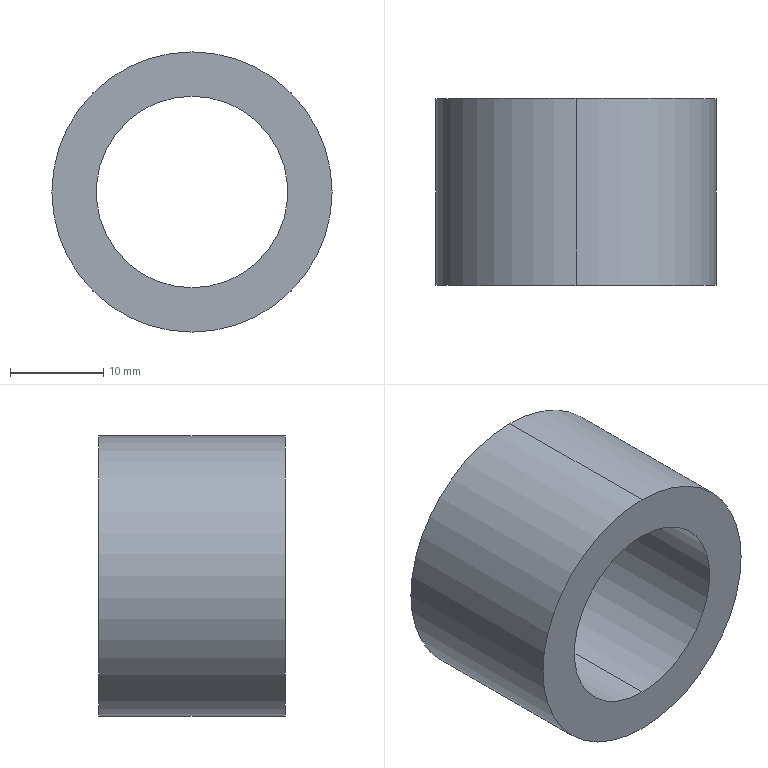Part | SolidWorks | features Extrusion 1 | 1 solid | 6 faces | box 30 x 20 x 30 mm | volume 7536 mm3 | cylinder 4 | plane 2 | commonest cylinder face diameters 20.5 x2 30 x2
STEP:
#1=CARTESIAN_POINT('',(0.,20.,-10.25));
#2=VERTEX_POINT('',#1);
#3=CARTESIAN_POINT('',(0.,20.,10.25));
#4=VERTEX_POINT('',#3);
#5=CARTESIAN_POINT('',(0.,20.,0.));
#6=DIRECTION('',(0.,1.,0.));
#7=DIRECTION('',(0.,0.,1.));
#8=AXIS2_PLACEMENT_3D('',#5,#6,#7);
#9=CIRCLE('',#8,10.25);
#10=EDGE_CURVE('',#2,#4,#9,.T.);
#11=ORIENTED_EDGE('',*,*,#10,.T.);
#12=CARTESIAN_POINT('',(0.,0.,10.25));
#13=VERTEX_POINT('',#12);
#14=CARTESIAN_POINT('',(0.,20.,10.25));
#15=DIRECTION('',(0.,-1.,0.));
#16=VECTOR('',#15,1000.);
#17=LINE('',#14,#16);
#18=EDGE_CURVE('',#4,#13,#17,.T.);
#19=ORIENTED_EDGE('',*,*,#18,.T.);
#20=CARTESIAN_POINT('',(0.,0.,-10.25));
#21=VERTEX_POINT('',#20);
#22=CARTESIAN_POINT('',(0.,0.,0.));
#23=DIRECTION('',(0.,1.,0.));
#24=DIRECTION('',(0.,0.,1.));
#25=AXIS2_PLACEMENT_3D('',#22,#23,#24);
#26=CIRCLE('',#25,10.25);
#27=EDGE_CURVE('',#21,#13,#26,.T.);
#28=ORIENTED_EDGE('',*,*,#27,.F.);
#29=CARTESIAN_POINT('',(0.,20.,-10.25));
#30=DIRECTION('',(0.,-1.,0.));
#31=VECTOR('',#30,1000.);
#32=LINE('',#29,#31);
#33=EDGE_CURVE('',#2,#21,#32,.T.);
#34=ORIENTED_EDGE('',*,*,#33,.F.);
#35=EDGE_LOOP('',(#11,#19,#28,#34));
#36=FACE_OUTER_BOUND('',#35,.T.);
#37=CARTESIAN_POINT('',(0.,20.,0.));
#38=DIRECTION('',(0.,-1.,0.));
#39=DIRECTION('',(0.,0.,-1.));
#40=AXIS2_PLACEMENT_3D('',#37,#38,#39);
#41=CYLINDRICAL_SURFACE('',#40,10.25);
#42=ADVANCED_FACE('',(#36),#41,.F.);
#43=CARTESIAN_POINT('',(0.,20.,15.));
#44=VERTEX_POINT('',#43);
#45=CARTESIAN_POINT('',(0.,20.,-15.));
#46=VERTEX_POINT('',#45);
#47=CARTESIAN_POINT('',(0.,20.,0.));
#48=DIRECTION('',(0.,1.,0.));
#49=DIRECTION('',(0.,0.,1.));
#50=AXIS2_PLACEMENT_3D('',#47,#48,#49);
#51=CIRCLE('',#50,15.);
#52=EDGE_CURVE('',#44,#46,#51,.T.);
#53=ORIENTED_EDGE('',*,*,#52,.F.);
#54=CARTESIAN_POINT('',(0.,0.,15.));
#55=VERTEX_POINT('',#54);
#56=CARTESIAN_POINT('',(0.,20.,15.));
#57=DIRECTION('',(0.,-1.,0.));
#58=VECTOR('',#57,1000.);
#59=LINE('',#56,#58);
#60=EDGE_CURVE('',#44,#55,#59,.T.);
#61=ORIENTED_EDGE('',*,*,#60,.T.);
#62=CARTESIAN_POINT('',(0.,0.,-15.));
#63=VERTEX_POINT('',#62);
#64=CARTESIAN_POINT('',(0.,0.,0.));
#65=DIRECTION('',(0.,1.,0.));
#66=DIRECTION('',(0.,0.,1.));
#67=AXIS2_PLACEMENT_3D('',#64,#65,#66);
#68=CIRCLE('',#67,15.);
#69=EDGE_CURVE('',#55,#63,#68,.T.);
#70=ORIENTED_EDGE('',*,*,#69,.T.);
#71=CARTESIAN_POINT('',(0.,20.,-15.));
#72=DIRECTION('',(0.,-1.,0.));
#73=VECTOR('',#72,1000.);
#74=LINE('',#71,#73);
#75=EDGE_CURVE('',#46,#63,#74,.T.);
#76=ORIENTED_EDGE('',*,*,#75,.F.);
#77=EDGE_LOOP('',(#53,#61,#70,#76));
#78=FACE_OUTER_BOUND('',#77,.T.);
#79=CARTESIAN_POINT('',(0.,20.,0.));
#80=DIRECTION('',(0.,-1.,0.));
#81=DIRECTION('',(0.,0.,-1.));
#82=AXIS2_PLACEMENT_3D('',#79,#80,#81);
#83=CYLINDRICAL_SURFACE('',#82,15.);
#84=ADVANCED_FACE('',(#78),#83,.T.);
#85=CARTESIAN_POINT('',(0.,20.,0.));
#86=DIRECTION('',(0.,1.,0.));
#87=DIRECTION('',(0.,0.,1.));
#88=AXIS2_PLACEMENT_3D('',#85,#86,#87);
#89=CIRCLE('',#88,15.);
#90=EDGE_CURVE('',#46,#44,#89,.T.);
#91=ORIENTED_EDGE('',*,*,#90,.T.);
#92=ORIENTED_EDGE('',*,*,#52,.T.);
#93=EDGE_LOOP('',(#91,#92));
#94=FACE_OUTER_BOUND('',#93,.T.);
#95=ORIENTED_EDGE('',*,*,#10,.F.);
#96=CARTESIAN_POINT('',(0.,20.,0.));
#97=DIRECTION('',(0.,1.,0.));
#98=DIRECTION('',(0.,0.,1.));
#99=AXIS2_PLACEMENT_3D('',#96,#97,#98);
#100=CIRCLE('',#99,10.25);
#101=EDGE_CURVE('',#4,#2,#100,.T.);
#102=ORIENTED_EDGE('',*,*,#101,.F.);
#103=EDGE_LOOP('',(#95,#102));
#104=FACE_BOUND('',#103,.T.);
#105=CARTESIAN_POINT('',(0.,20.,0.));
#106=DIRECTION('',(0.,1.,0.));
#107=DIRECTION('',(0.,0.,1.));
#108=AXIS2_PLACEMENT_3D('',#105,#106,#107);
#109=PLANE('',#108);
#110=ADVANCED_FACE('',(#94,#104),#109,.T.);
#111=CARTESIAN_POINT('',(0.,0.,0.));
#112=DIRECTION('',(0.,1.,0.));
#113=DIRECTION('',(0.,0.,1.));
#114=AXIS2_PLACEMENT_3D('',#111,#112,#113);
#115=CIRCLE('',#114,15.);
#116=EDGE_CURVE('',#63,#55,#115,.T.);
#117=ORIENTED_EDGE('',*,*,#116,.F.);
#118=ORIENTED_EDGE('',*,*,#69,.F.);
#119=EDGE_LOOP('',(#117,#118));
#120=FACE_OUTER_BOUND('',#119,.T.);
#121=ORIENTED_EDGE('',*,*,#27,.T.);
#122=CARTESIAN_POINT('',(0.,0.,0.));
#123=DIRECTION('',(0.,1.,0.));
#124=DIRECTION('',(0.,0.,1.));
#125=AXIS2_PLACEMENT_3D('',#122,#123,#124);
#126=CIRCLE('',#125,10.25);
#127=EDGE_CURVE('',#13,#21,#126,.T.);
#128=ORIENTED_EDGE('',*,*,#127,.T.);
#129=EDGE_LOOP('',(#121,#128));
#130=FACE_BOUND('',#129,.T.);
#131=CARTESIAN_POINT('',(0.,0.,0.));
#132=DIRECTION('',(0.,1.,0.));
#133=DIRECTION('',(0.,0.,1.));
#134=AXIS2_PLACEMENT_3D('',#131,#132,#133);
#135=PLANE('',#134);
#136=ADVANCED_FACE('',(#120,#130),#135,.F.);
#137=ORIENTED_EDGE('',*,*,#60,.F.);
#138=ORIENTED_EDGE('',*,*,#90,.F.);
#139=ORIENTED_EDGE('',*,*,#75,.T.);
#140=ORIENTED_EDGE('',*,*,#116,.T.);
#141=EDGE_LOOP('',(#137,#138,#139,#140));
#142=FACE_OUTER_BOUND('',#141,.T.);
#143=CARTESIAN_POINT('',(0.,20.,0.));
#144=DIRECTION('',(0.,-1.,0.));
#145=DIRECTION('',(0.,0.,-1.));
#146=AXIS2_PLACEMENT_3D('',#143,#144,#145);
#147=CYLINDRICAL_SURFACE('',#146,15.);
#148=ADVANCED_FACE('',(#142),#147,.T.);
#149=ORIENTED_EDGE('',*,*,#18,.F.);
#150=ORIENTED_EDGE('',*,*,#101,.T.);
#151=ORIENTED_EDGE('',*,*,#33,.T.);
#152=ORIENTED_EDGE('',*,*,#127,.F.);
#153=EDGE_LOOP('',(#149,#150,#151,#152));
#154=FACE_OUTER_BOUND('',#153,.T.);
#155=CARTESIAN_POINT('',(0.,20.,0.));
#156=DIRECTION('',(0.,-1.,0.));
#157=DIRECTION('',(0.,0.,-1.));
#158=AXIS2_PLACEMENT_3D('',#155,#156,#157);
#159=CYLINDRICAL_SURFACE('',#158,10.25);
#160=ADVANCED_FACE('',(#154),#159,.F.);
#161=CLOSED_SHELL('',(#42,#84,#110,#136,#148,#160));
#162=MANIFOLD_SOLID_BREP('',#161);
#163=CARTESIAN_POINT('',(0.,0.,0.));
#164=DIRECTION('',(0.,0.,1.));
#165=DIRECTION('',(1.,0.,0.));
#166=AXIS2_PLACEMENT_3D('',#163,#164,#165);
#167=(LENGTH_UNIT()NAMED_UNIT(*)SI_UNIT(.MILLI.,.METRE.));
#168=UNCERTAINTY_MEASURE_WITH_UNIT(LENGTH_MEASURE(0.00001),#167,'','');
#169=(NAMED_UNIT(*)PLANE_ANGLE_UNIT()SI_UNIT($,.RADIAN.));
#170=(NAMED_UNIT(*)SI_UNIT($,.STERADIAN.)SOLID_ANGLE_UNIT());
#171=(GEOMETRIC_REPRESENTATION_CONTEXT(3)GLOBAL_UNCERTAINTY_ASSIGNED_CONTEXT((#168))GLOBAL_UNIT_ASSIGNED_CONTEXT((#167,#169,#170))REPRESENTATION_CONTEXT('',''));
#172=ADVANCED_BREP_SHAPE_REPRESENTATION('',(#162,#166),#171);